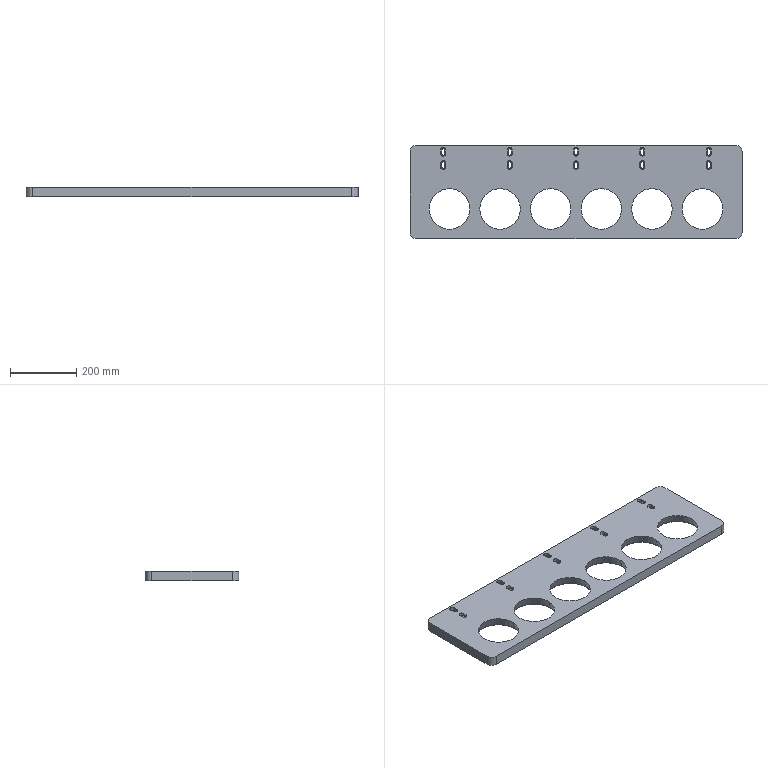Part | SolidWorks | features BaseBody 1 | 1 solid | 124 faces | box 1000 x 282 x 30 mm | volume 5952206 mm3 | plane 56 | cylinder 44 | torus 12 | cone 12 | commonest cylinder face diameters 9 x20 15 x20 40 x4